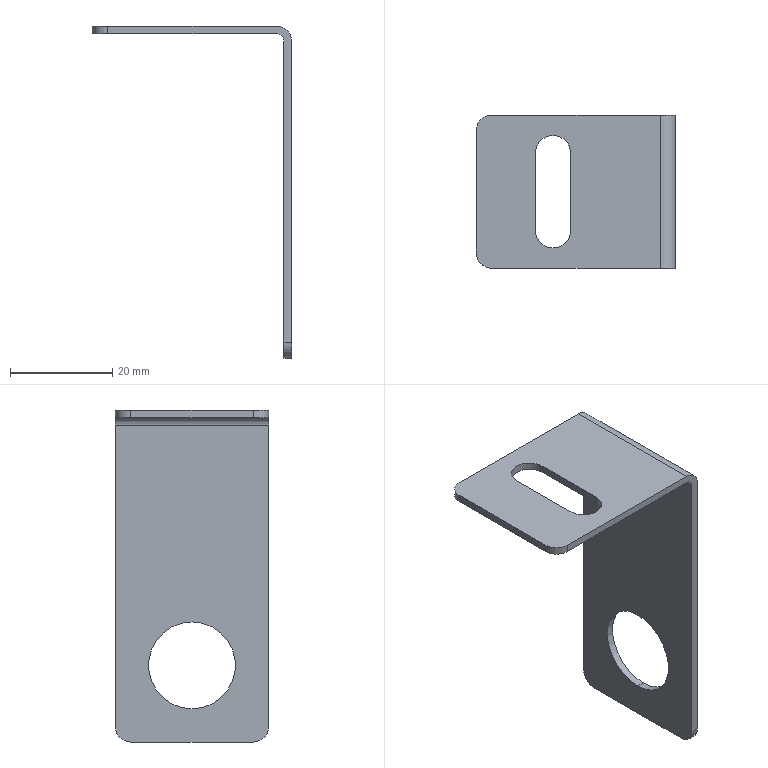Part | SolidWorks | features BaseBody 1 | 1 solid | 20 faces | box 39 x 30 x 65 mm | volume 4002 mm3 | cylinder 10 | plane 10 | commonest cylinder face diameters 6 x5 7 x2 17 x2 3 x1
STEP:
#1=CARTESIAN_POINT('',(18.,0.,-58.5));
#2=VERTEX_POINT('',#1);
#3=CARTESIAN_POINT('',(18.,0.,-41.5));
#4=VERTEX_POINT('',#3);
#5=CARTESIAN_POINT('',(18.,0.,-50.));
#6=DIRECTION('',(-1.,0.,0.));
#7=DIRECTION('',(0.,0.,-1.));
#8=AXIS2_PLACEMENT_3D('',#5,#6,#7);
#9=CIRCLE('',#8,8.5);
#10=EDGE_CURVE('',#2,#4,#9,.T.);
#11=ORIENTED_EDGE('',*,*,#10,.T.);
#12=CARTESIAN_POINT('',(19.5,0.,-41.5));
#13=VERTEX_POINT('',#12);
#14=CARTESIAN_POINT('',(9.5,0.,-41.5));
#15=DIRECTION('',(1.,0.,0.));
#16=VECTOR('',#15,1000.);
#17=LINE('',#14,#16);
#18=EDGE_CURVE('',#4,#13,#17,.T.);
#19=ORIENTED_EDGE('',*,*,#18,.T.);
#20=CARTESIAN_POINT('',(19.5,0.,-58.5));
#21=VERTEX_POINT('',#20);
#22=CARTESIAN_POINT('',(19.5,0.,-50.));
#23=DIRECTION('',(-1.,0.,0.));
#24=DIRECTION('',(0.,0.,-1.));
#25=AXIS2_PLACEMENT_3D('',#22,#23,#24);
#26=CIRCLE('',#25,8.5);
#27=EDGE_CURVE('',#21,#13,#26,.T.);
#28=ORIENTED_EDGE('',*,*,#27,.F.);
#29=CARTESIAN_POINT('',(9.5,0.,-58.5));
#30=DIRECTION('',(1.,0.,0.));
#31=VECTOR('',#30,1000.);
#32=LINE('',#29,#31);
#33=EDGE_CURVE('',#2,#21,#32,.T.);
#34=ORIENTED_EDGE('',*,*,#33,.F.);
#35=EDGE_LOOP('',(#11,#19,#28,#34));
#36=FACE_OUTER_BOUND('',#35,.T.);
#37=CARTESIAN_POINT('',(9.5,0.,-50.));
#38=DIRECTION('',(1.,0.,0.));
#39=DIRECTION('',(0.,0.,-1.));
#40=AXIS2_PLACEMENT_3D('',#37,#38,#39);
#41=CYLINDRICAL_SURFACE('',#40,8.5);
#42=ADVANCED_FACE('',(#36),#41,.F.);
#43=CARTESIAN_POINT('',(18.,12.,-65.));
#44=VERTEX_POINT('',#43);
#45=CARTESIAN_POINT('',(18.,15.,-62.));
#46=VERTEX_POINT('',#45);
#47=CARTESIAN_POINT('',(18.,12.,-62.));
#48=DIRECTION('',(1.,0.,0.));
#49=DIRECTION('',(0.,0.,1.));
#50=AXIS2_PLACEMENT_3D('',#47,#48,#49);
#51=CIRCLE('',#50,3.);
#52=EDGE_CURVE('',#44,#46,#51,.T.);
#53=ORIENTED_EDGE('',*,*,#52,.F.);
#54=CARTESIAN_POINT('',(18.,-12.,-65.));
#55=VERTEX_POINT('',#54);
#56=CARTESIAN_POINT('',(18.,0.,-65.));
#57=DIRECTION('',(0.,1.,0.));
#58=VECTOR('',#57,1000.);
#59=LINE('',#56,#58);
#60=EDGE_CURVE('',#55,#44,#59,.T.);
#61=ORIENTED_EDGE('',*,*,#60,.F.);
#62=CARTESIAN_POINT('',(18.,-15.,-62.));
#63=VERTEX_POINT('',#62);
#64=CARTESIAN_POINT('',(18.,-12.,-62.));
#65=DIRECTION('',(1.,0.,0.));
#66=DIRECTION('',(0.,0.,1.));
#67=AXIS2_PLACEMENT_3D('',#64,#65,#66);
#68=CIRCLE('',#67,3.);
#69=EDGE_CURVE('',#63,#55,#68,.T.);
#70=ORIENTED_EDGE('',*,*,#69,.F.);
#71=CARTESIAN_POINT('',(18.,-15.,-3.));
#72=VERTEX_POINT('',#71);
#73=CARTESIAN_POINT('',(18.,-15.,0.));
#74=DIRECTION('',(0.,0.,-1.));
#75=VECTOR('',#74,1000.);
#76=LINE('',#73,#75);
#77=EDGE_CURVE('',#72,#63,#76,.T.);
#78=ORIENTED_EDGE('',*,*,#77,.F.);
#79=CARTESIAN_POINT('',(18.,15.,-3.));
#80=VERTEX_POINT('',#79);
#81=CARTESIAN_POINT('',(18.,0.,-3.));
#82=DIRECTION('',(0.,-1.,0.));
#83=VECTOR('',#82,1000.);
#84=LINE('',#81,#83);
#85=EDGE_CURVE('',#80,#72,#84,.T.);
#86=ORIENTED_EDGE('',*,*,#85,.F.);
#87=CARTESIAN_POINT('',(18.,15.,0.));
#88=DIRECTION('',(0.,0.,1.));
#89=VECTOR('',#88,1000.);
#90=LINE('',#87,#89);
#91=EDGE_CURVE('',#46,#80,#90,.T.);
#92=ORIENTED_EDGE('',*,*,#91,.F.);
#93=EDGE_LOOP('',(#53,#61,#70,#78,#86,#92));
#94=FACE_OUTER_BOUND('',#93,.T.);
#95=ORIENTED_EDGE('',*,*,#10,.F.);
#96=CARTESIAN_POINT('',(18.,0.,-50.));
#97=DIRECTION('',(-1.,0.,0.));
#98=DIRECTION('',(0.,0.,-1.));
#99=AXIS2_PLACEMENT_3D('',#96,#97,#98);
#100=CIRCLE('',#99,8.5);
#101=EDGE_CURVE('',#4,#2,#100,.T.);
#102=ORIENTED_EDGE('',*,*,#101,.F.);
#103=EDGE_LOOP('',(#95,#102));
#104=FACE_BOUND('',#103,.T.);
#105=CARTESIAN_POINT('',(18.,0.,0.));
#106=DIRECTION('',(1.,0.,0.));
#107=DIRECTION('',(0.,0.,-1.));
#108=AXIS2_PLACEMENT_3D('',#105,#106,#107);
#109=PLANE('',#108);
#110=ADVANCED_FACE('',(#94,#104),#109,.F.);
#111=ORIENTED_EDGE('',*,*,#91,.T.);
#112=CARTESIAN_POINT('',(16.5,15.,-1.5));
#113=VERTEX_POINT('',#112);
#114=CARTESIAN_POINT('',(16.5,15.,-3.));
#115=DIRECTION('',(0.,-1.,0.));
#116=DIRECTION('',(0.,0.,-1.));
#117=AXIS2_PLACEMENT_3D('',#114,#115,#116);
#118=CIRCLE('',#117,1.5);
#119=EDGE_CURVE('',#80,#113,#118,.T.);
#120=ORIENTED_EDGE('',*,*,#119,.T.);
#121=CARTESIAN_POINT('',(-16.5,15.,-1.5));
#122=VERTEX_POINT('',#121);
#123=CARTESIAN_POINT('',(0.,15.,-1.5));
#124=DIRECTION('',(1.,0.,0.));
#125=VECTOR('',#124,1000.);
#126=LINE('',#123,#125);
#127=EDGE_CURVE('',#122,#113,#126,.T.);
#128=ORIENTED_EDGE('',*,*,#127,.F.);
#129=CARTESIAN_POINT('',(-16.5,15.,0.));
#130=VERTEX_POINT('',#129);
#131=CARTESIAN_POINT('',(-16.5,15.,-1.5));
#132=DIRECTION('',(0.,0.,1.));
#133=VECTOR('',#132,1000.);
#134=LINE('',#131,#133);
#135=EDGE_CURVE('',#122,#130,#134,.T.);
#136=ORIENTED_EDGE('',*,*,#135,.T.);
#137=CARTESIAN_POINT('',(16.5,15.,0.));
#138=VERTEX_POINT('',#137);
#139=CARTESIAN_POINT('',(-19.5,15.,0.));
#140=DIRECTION('',(1.,0.,0.));
#141=VECTOR('',#140,1000.);
#142=LINE('',#139,#141);
#143=EDGE_CURVE('',#130,#138,#142,.T.);
#144=ORIENTED_EDGE('',*,*,#143,.T.);
#145=CARTESIAN_POINT('',(19.5,15.,-3.));
#146=VERTEX_POINT('',#145);
#147=CARTESIAN_POINT('',(16.5,15.,-3.));
#148=DIRECTION('',(0.,1.,0.));
#149=DIRECTION('',(0.,0.,-1.));
#150=AXIS2_PLACEMENT_3D('',#147,#148,#149);
#151=CIRCLE('',#150,3.);
#152=EDGE_CURVE('',#138,#146,#151,.T.);
#153=ORIENTED_EDGE('',*,*,#152,.T.);
#154=CARTESIAN_POINT('',(19.5,15.,-62.));
#155=VERTEX_POINT('',#154);
#156=CARTESIAN_POINT('',(19.5,15.,-65.));
#157=DIRECTION('',(0.,0.,-1.));
#158=VECTOR('',#157,1000.);
#159=LINE('',#156,#158);
#160=EDGE_CURVE('',#146,#155,#159,.T.);
#161=ORIENTED_EDGE('',*,*,#160,.T.);
#162=CARTESIAN_POINT('',(19.5,15.,-62.));
#163=DIRECTION('',(-1.,0.,0.));
#164=VECTOR('',#163,1000.);
#165=LINE('',#162,#164);
#166=EDGE_CURVE('',#155,#46,#165,.T.);
#167=ORIENTED_EDGE('',*,*,#166,.T.);
#168=EDGE_LOOP('',(#111,#120,#128,#136,#144,#153,#161,#167));
#169=FACE_OUTER_BOUND('',#168,.T.);
#170=CARTESIAN_POINT('',(19.5,15.,-65.));
#171=DIRECTION('',(0.,1.,0.));
#172=DIRECTION('',(0.,0.,1.));
#173=AXIS2_PLACEMENT_3D('',#170,#171,#172);
#174=PLANE('',#173);
#175=ADVANCED_FACE('',(#169),#174,.T.);
#176=ORIENTED_EDGE('',*,*,#52,.T.);
#177=ORIENTED_EDGE('',*,*,#166,.F.);
#178=CARTESIAN_POINT('',(19.5,12.,-65.));
#179=VERTEX_POINT('',#178);
#180=CARTESIAN_POINT('',(19.5,12.,-62.));
#181=DIRECTION('',(-1.,0.,0.));
#182=DIRECTION('',(0.,0.,1.));
#183=AXIS2_PLACEMENT_3D('',#180,#181,#182);
#184=CIRCLE('',#183,3.);
#185=EDGE_CURVE('',#155,#179,#184,.T.);
#186=ORIENTED_EDGE('',*,*,#185,.T.);
#187=CARTESIAN_POINT('',(19.5,12.,-65.));
#188=DIRECTION('',(-1.,0.,0.));
#189=VECTOR('',#188,1000.);
#190=LINE('',#187,#189);
#191=EDGE_CURVE('',#179,#44,#190,.T.);
#192=ORIENTED_EDGE('',*,*,#191,.T.);
#193=EDGE_LOOP('',(#176,#177,#186,#192));
#194=FACE_OUTER_BOUND('',#193,.T.);
#195=CARTESIAN_POINT('',(19.5,12.,-62.));
#196=DIRECTION('',(-1.,0.,0.));
#197=DIRECTION('',(0.,0.,1.));
#198=AXIS2_PLACEMENT_3D('',#195,#196,#197);
#199=CYLINDRICAL_SURFACE('',#198,3.);
#200=ADVANCED_FACE('',(#194),#199,.T.);
#201=CARTESIAN_POINT('',(19.5,-12.,-65.));
#202=VERTEX_POINT('',#201);
#203=CARTESIAN_POINT('',(19.5,-15.,-65.));
#204=DIRECTION('',(0.,-1.,0.));
#205=VECTOR('',#204,1000.);
#206=LINE('',#203,#205);
#207=EDGE_CURVE('',#179,#202,#206,.T.);
#208=ORIENTED_EDGE('',*,*,#207,.T.);
#209=CARTESIAN_POINT('',(19.5,-12.,-65.));
#210=DIRECTION('',(-1.,0.,0.));
#211=VECTOR('',#210,1000.);
#212=LINE('',#209,#211);
#213=EDGE_CURVE('',#202,#55,#212,.T.);
#214=ORIENTED_EDGE('',*,*,#213,.T.);
#215=ORIENTED_EDGE('',*,*,#60,.T.);
#216=ORIENTED_EDGE('',*,*,#191,.F.);
#217=EDGE_LOOP('',(#208,#214,#215,#216));
#218=FACE_OUTER_BOUND('',#217,.T.);
#219=CARTESIAN_POINT('',(19.5,-15.,-65.));
#220=DIRECTION('',(0.,0.,-1.));
#221=DIRECTION('',(-1.,0.,0.));
#222=AXIS2_PLACEMENT_3D('',#219,#220,#221);
#223=PLANE('',#222);
#224=ADVANCED_FACE('',(#218),#223,.T.);
#225=ORIENTED_EDGE('',*,*,#69,.T.);
#226=ORIENTED_EDGE('',*,*,#213,.F.);
#227=CARTESIAN_POINT('',(19.5,-15.,-62.));
#228=VERTEX_POINT('',#227);
#229=CARTESIAN_POINT('',(19.5,-12.,-62.));
#230=DIRECTION('',(-1.,0.,0.));
#231=DIRECTION('',(0.,0.,1.));
#232=AXIS2_PLACEMENT_3D('',#229,#230,#231);
#233=CIRCLE('',#232,3.);
#234=EDGE_CURVE('',#202,#228,#233,.T.);
#235=ORIENTED_EDGE('',*,*,#234,.T.);
#236=CARTESIAN_POINT('',(19.5,-15.,-62.));
#237=DIRECTION('',(-1.,0.,0.));
#238=VECTOR('',#237,1000.);
#239=LINE('',#236,#238);
#240=EDGE_CURVE('',#228,#63,#239,.T.);
#241=ORIENTED_EDGE('',*,*,#240,.T.);
#242=EDGE_LOOP('',(#225,#226,#235,#241));
#243=FACE_OUTER_BOUND('',#242,.T.);
#244=CARTESIAN_POINT('',(19.5,-12.,-62.));
#245=DIRECTION('',(-1.,0.,0.));
#246=DIRECTION('',(0.,0.,1.));
#247=AXIS2_PLACEMENT_3D('',#244,#245,#246);
#248=CYLINDRICAL_SURFACE('',#247,3.);
#249=ADVANCED_FACE('',(#243),#248,.T.);
#250=CARTESIAN_POINT('',(19.5,-15.,-3.));
#251=VERTEX_POINT('',#250);
#252=CARTESIAN_POINT('',(19.5,-15.,-1.5));
#253=DIRECTION('',(0.,0.,1.));
#254=VECTOR('',#253,1000.);
#255=LINE('',#252,#254);
#256=EDGE_CURVE('',#228,#251,#255,.T.);
#257=ORIENTED_EDGE('',*,*,#256,.T.);
#258=CARTESIAN_POINT('',(16.5,-15.,0.));
#259=VERTEX_POINT('',#258);
#260=CARTESIAN_POINT('',(16.5,-15.,-3.));
#261=DIRECTION('',(0.,1.,0.));
#262=DIRECTION('',(0.,0.,-1.));
#263=AXIS2_PLACEMENT_3D('',#260,#261,#262);
#264=CIRCLE('',#263,3.);
#265=EDGE_CURVE('',#259,#251,#264,.T.);
#266=ORIENTED_EDGE('',*,*,#265,.F.);
#267=CARTESIAN_POINT('',(-16.5,-15.,0.));
#268=VERTEX_POINT('',#267);
#269=CARTESIAN_POINT('',(-19.5,-15.,0.));
#270=DIRECTION('',(-1.,0.,0.));
#271=VECTOR('',#270,1000.);
#272=LINE('',#269,#271);
#273=EDGE_CURVE('',#259,#268,#272,.T.);
#274=ORIENTED_EDGE('',*,*,#273,.T.);
#275=CARTESIAN_POINT('',(-16.5,-15.,-1.5));
#276=VERTEX_POINT('',#275);
#277=CARTESIAN_POINT('',(-16.5,-15.,-1.5));
#278=DIRECTION('',(0.,0.,1.));
#279=VECTOR('',#278,1000.);
#280=LINE('',#277,#279);
#281=EDGE_CURVE('',#276,#268,#280,.T.);
#282=ORIENTED_EDGE('',*,*,#281,.F.);
#283=CARTESIAN_POINT('',(16.5,-15.,-1.5));
#284=VERTEX_POINT('',#283);
#285=CARTESIAN_POINT('',(0.,-15.,-1.5));
#286=DIRECTION('',(-1.,0.,0.));
#287=VECTOR('',#286,1000.);
#288=LINE('',#285,#287);
#289=EDGE_CURVE('',#284,#276,#288,.T.);
#290=ORIENTED_EDGE('',*,*,#289,.F.);
#291=CARTESIAN_POINT('',(16.5,-15.,-3.));
#292=DIRECTION('',(0.,1.,0.));
#293=DIRECTION('',(0.,0.,-1.));
#294=AXIS2_PLACEMENT_3D('',#291,#292,#293);
#295=CIRCLE('',#294,1.5);
#296=EDGE_CURVE('',#284,#72,#295,.T.);
#297=ORIENTED_EDGE('',*,*,#296,.T.);
#298=ORIENTED_EDGE('',*,*,#77,.T.);
#299=ORIENTED_EDGE('',*,*,#240,.F.);
#300=EDGE_LOOP('',(#257,#266,#274,#282,#290,#297,#298,#299));
#301=FACE_OUTER_BOUND('',#300,.T.);
#302=CARTESIAN_POINT('',(19.5,-15.,-1.5));
#303=DIRECTION('',(0.,-1.,0.));
#304=DIRECTION('',(0.,0.,-1.));
#305=AXIS2_PLACEMENT_3D('',#302,#303,#304);
#306=PLANE('',#305);
#307=ADVANCED_FACE('',(#301),#306,.T.);
#308=ORIENTED_EDGE('',*,*,#119,.F.);
#309=ORIENTED_EDGE('',*,*,#85,.T.);
#310=ORIENTED_EDGE('',*,*,#296,.F.);
#311=CARTESIAN_POINT('',(16.5,-15.,-1.5));
#312=DIRECTION('',(0.,-1.,0.));
#313=VECTOR('',#312,1000.);
#314=LINE('',#311,#313);
#315=EDGE_CURVE('',#113,#284,#314,.T.);
#316=ORIENTED_EDGE('',*,*,#315,.F.);
#317=EDGE_LOOP('',(#308,#309,#310,#316));
#318=FACE_OUTER_BOUND('',#317,.T.);
#319=CARTESIAN_POINT('',(16.5,-15.,-3.));
#320=DIRECTION('',(0.,-1.,0.));
#321=DIRECTION('',(0.,0.,-1.));
#322=AXIS2_PLACEMENT_3D('',#319,#320,#321);
#323=CYLINDRICAL_SURFACE('',#322,1.5);
#324=ADVANCED_FACE('',(#318),#323,.F.);
#325=ORIENTED_EDGE('',*,*,#18,.F.);
#326=ORIENTED_EDGE('',*,*,#101,.T.);
#327=ORIENTED_EDGE('',*,*,#33,.T.);
#328=CARTESIAN_POINT('',(19.5,0.,-50.));
#329=DIRECTION('',(-1.,0.,0.));
#330=DIRECTION('',(0.,0.,-1.));
#331=AXIS2_PLACEMENT_3D('',#328,#329,#330);
#332=CIRCLE('',#331,8.5);
#333=EDGE_CURVE('',#13,#21,#332,.T.);
#334=ORIENTED_EDGE('',*,*,#333,.F.);
#335=EDGE_LOOP('',(#325,#326,#327,#334));
#336=FACE_OUTER_BOUND('',#335,.T.);
#337=CARTESIAN_POINT('',(9.5,0.,-50.));
#338=DIRECTION('',(1.,0.,0.));
#339=DIRECTION('',(0.,0.,-1.));
#340=AXIS2_PLACEMENT_3D('',#337,#338,#339);
#341=CYLINDRICAL_SURFACE('',#340,8.5);
#342=ADVANCED_FACE('',(#336),#341,.F.);
#343=ORIENTED_EDGE('',*,*,#256,.F.);
#344=ORIENTED_EDGE('',*,*,#234,.F.);
#345=ORIENTED_EDGE('',*,*,#207,.F.);
#346=ORIENTED_EDGE('',*,*,#185,.F.);
#347=ORIENTED_EDGE('',*,*,#160,.F.);
#348=CARTESIAN_POINT('',(19.5,0.,-3.));
#349=DIRECTION('',(0.,-1.,0.));
#350=VECTOR('',#349,1000.);
#351=LINE('',#348,#350);
#352=EDGE_CURVE('',#146,#251,#351,.T.);
#353=ORIENTED_EDGE('',*,*,#352,.T.);
#354=EDGE_LOOP('',(#343,#344,#345,#346,#347,#353));
#355=FACE_OUTER_BOUND('',#354,.T.);
#356=ORIENTED_EDGE('',*,*,#27,.T.);
#357=ORIENTED_EDGE('',*,*,#333,.T.);
#358=EDGE_LOOP('',(#356,#357));
#359=FACE_BOUND('',#358,.T.);
#360=CARTESIAN_POINT('',(19.5,0.,0.));
#361=DIRECTION('',(1.,0.,0.));
#362=DIRECTION('',(0.,0.,-1.));
#363=AXIS2_PLACEMENT_3D('',#360,#361,#362);
#364=PLANE('',#363);
#365=ADVANCED_FACE('',(#355,#359),#364,.T.);
#366=ORIENTED_EDGE('',*,*,#289,.T.);
#367=CARTESIAN_POINT('',(-19.5,-12.,-1.5));
#368=VERTEX_POINT('',#367);
#369=CARTESIAN_POINT('',(-16.5,-12.,-1.5));
#370=DIRECTION('',(0.,0.,-1.));
#371=DIRECTION('',(1.,0.,0.));
#372=AXIS2_PLACEMENT_3D('',#369,#370,#371);
#373=CIRCLE('',#372,3.);
#374=EDGE_CURVE('',#276,#368,#373,.T.);
#375=ORIENTED_EDGE('',*,*,#374,.T.);
#376=CARTESIAN_POINT('',(-19.5,12.,-1.5));
#377=VERTEX_POINT('',#376);
#378=CARTESIAN_POINT('',(-19.5,0.,-1.5));
#379=DIRECTION('',(0.,1.,0.));
#380=VECTOR('',#379,1000.);
#381=LINE('',#378,#380);
#382=EDGE_CURVE('',#368,#377,#381,.T.);
#383=ORIENTED_EDGE('',*,*,#382,.T.);
#384=CARTESIAN_POINT('',(-16.5,12.,-1.5));
#385=DIRECTION('',(0.,0.,-1.));
#386=DIRECTION('',(1.,0.,0.));
#387=AXIS2_PLACEMENT_3D('',#384,#385,#386);
#388=CIRCLE('',#387,3.);
#389=EDGE_CURVE('',#377,#122,#388,.T.);
#390=ORIENTED_EDGE('',*,*,#389,.T.);
#391=ORIENTED_EDGE('',*,*,#127,.T.);
#392=ORIENTED_EDGE('',*,*,#315,.T.);
#393=EDGE_LOOP('',(#366,#375,#383,#390,#391,#392));
#394=FACE_OUTER_BOUND('',#393,.T.);
#395=CARTESIAN_POINT('',(-8.,-7.5,-1.5));
#396=VERTEX_POINT('',#395);
#397=CARTESIAN_POINT('',(-1.,-7.5,-1.5));
#398=VERTEX_POINT('',#397);
#399=CARTESIAN_POINT('',(-4.5,-7.5,-1.5));
#400=DIRECTION('',(0.,0.,1.));
#401=DIRECTION('',(1.,0.,0.));
#402=AXIS2_PLACEMENT_3D('',#399,#400,#401);
#403=CIRCLE('',#402,3.5);
#404=EDGE_CURVE('',#396,#398,#403,.T.);
#405=ORIENTED_EDGE('',*,*,#404,.T.);
#406=CARTESIAN_POINT('',(-1.,7.5,-1.5));
#407=VERTEX_POINT('',#406);
#408=CARTESIAN_POINT('',(-1.,0.,-1.5));
#409=DIRECTION('',(0.,1.,0.));
#410=VECTOR('',#409,1000.);
#411=LINE('',#408,#410);
#412=EDGE_CURVE('',#398,#407,#411,.T.);
#413=ORIENTED_EDGE('',*,*,#412,.T.);
#414=CARTESIAN_POINT('',(-8.,7.5,-1.5));
#415=VERTEX_POINT('',#414);
#416=CARTESIAN_POINT('',(-4.5,7.5,-1.5));
#417=DIRECTION('',(0.,0.,1.));
#418=DIRECTION('',(1.,0.,0.));
#419=AXIS2_PLACEMENT_3D('',#416,#417,#418);
#420=CIRCLE('',#419,3.5);
#421=EDGE_CURVE('',#407,#415,#420,.T.);
#422=ORIENTED_EDGE('',*,*,#421,.T.);
#423=CARTESIAN_POINT('',(-8.,0.,-1.5));
#424=DIRECTION('',(0.,-1.,0.));
#425=VECTOR('',#424,1000.);
#426=LINE('',#423,#425);
#427=EDGE_CURVE('',#415,#396,#426,.T.);
#428=ORIENTED_EDGE('',*,*,#427,.T.);
#429=EDGE_LOOP('',(#405,#413,#422,#428));
#430=FACE_BOUND('',#429,.T.);
#431=CARTESIAN_POINT('',(0.,0.,-1.5));
#432=DIRECTION('',(0.,0.,-1.));
#433=DIRECTION('',(-1.,0.,0.));
#434=AXIS2_PLACEMENT_3D('',#431,#432,#433);
#435=PLANE('',#434);
#436=ADVANCED_FACE('',(#394,#430),#435,.T.);
#437=ORIENTED_EDGE('',*,*,#352,.F.);
#438=ORIENTED_EDGE('',*,*,#152,.F.);
#439=CARTESIAN_POINT('',(16.5,-15.,0.));
#440=DIRECTION('',(0.,-1.,0.));
#441=VECTOR('',#440,1000.);
#442=LINE('',#439,#441);
#443=EDGE_CURVE('',#138,#259,#442,.T.);
#444=ORIENTED_EDGE('',*,*,#443,.T.);
#445=ORIENTED_EDGE('',*,*,#265,.T.);
#446=EDGE_LOOP('',(#437,#438,#444,#445));
#447=FACE_OUTER_BOUND('',#446,.T.);
#448=CARTESIAN_POINT('',(16.5,-15.,-3.));
#449=DIRECTION('',(0.,-1.,0.));
#450=DIRECTION('',(0.,0.,-1.));
#451=AXIS2_PLACEMENT_3D('',#448,#449,#450);
#452=CYLINDRICAL_SURFACE('',#451,3.);
#453=ADVANCED_FACE('',(#447),#452,.T.);
#454=CARTESIAN_POINT('',(-19.5,-12.,0.));
#455=VERTEX_POINT('',#454);
#456=CARTESIAN_POINT('',(-16.5,-12.,0.));
#457=DIRECTION('',(0.,0.,-1.));
#458=DIRECTION('',(1.,0.,0.));
#459=AXIS2_PLACEMENT_3D('',#456,#457,#458);
#460=CIRCLE('',#459,3.);
#461=EDGE_CURVE('',#268,#455,#460,.T.);
#462=ORIENTED_EDGE('',*,*,#461,.T.);
#463=CARTESIAN_POINT('',(-19.5,-12.,-1.5));
#464=DIRECTION('',(0.,0.,-1.));
#465=VECTOR('',#464,1000.);
#466=LINE('',#463,#465);
#467=EDGE_CURVE('',#455,#368,#466,.T.);
#468=ORIENTED_EDGE('',*,*,#467,.T.);
#469=ORIENTED_EDGE('',*,*,#374,.F.);
#470=ORIENTED_EDGE('',*,*,#281,.T.);
#471=EDGE_LOOP('',(#462,#468,#469,#470));
#472=FACE_OUTER_BOUND('',#471,.T.);
#473=CARTESIAN_POINT('',(-16.5,-12.,-1.5));
#474=DIRECTION('',(0.,0.,1.));
#475=DIRECTION('',(1.,0.,0.));
#476=AXIS2_PLACEMENT_3D('',#473,#474,#475);
#477=CYLINDRICAL_SURFACE('',#476,3.);
#478=ADVANCED_FACE('',(#472),#477,.T.);
#479=CARTESIAN_POINT('',(-19.5,12.,0.));
#480=VERTEX_POINT('',#479);
#481=CARTESIAN_POINT('',(-16.5,12.,0.));
#482=DIRECTION('',(0.,0.,-1.));
#483=DIRECTION('',(1.,0.,0.));
#484=AXIS2_PLACEMENT_3D('',#481,#482,#483);
#485=CIRCLE('',#484,3.);
#486=EDGE_CURVE('',#480,#130,#485,.T.);
#487=ORIENTED_EDGE('',*,*,#486,.T.);
#488=ORIENTED_EDGE('',*,*,#135,.F.);
#489=ORIENTED_EDGE('',*,*,#389,.F.);
#490=CARTESIAN_POINT('',(-19.5,12.,-1.5));
#491=DIRECTION('',(0.,0.,1.));
#492=VECTOR('',#491,1000.);
#493=LINE('',#490,#492);
#494=EDGE_CURVE('',#377,#480,#493,.T.);
#495=ORIENTED_EDGE('',*,*,#494,.T.);
#496=EDGE_LOOP('',(#487,#488,#489,#495));
#497=FACE_OUTER_BOUND('',#496,.T.);
#498=CARTESIAN_POINT('',(-16.5,12.,-1.5));
#499=DIRECTION('',(0.,0.,1.));
#500=DIRECTION('',(1.,0.,0.));
#501=AXIS2_PLACEMENT_3D('',#498,#499,#500);
#502=CYLINDRICAL_SURFACE('',#501,3.);
#503=ADVANCED_FACE('',(#497),#502,.T.);
#504=ORIENTED_EDGE('',*,*,#382,.F.);
#505=ORIENTED_EDGE('',*,*,#467,.F.);
#506=CARTESIAN_POINT('',(-19.5,-15.,0.));
#507=DIRECTION('',(0.,1.,0.));
#508=VECTOR('',#507,1000.);
#509=LINE('',#506,#508);
#510=EDGE_CURVE('',#455,#480,#509,.T.);
#511=ORIENTED_EDGE('',*,*,#510,.T.);
#512=ORIENTED_EDGE('',*,*,#494,.F.);
#513=EDGE_LOOP('',(#504,#505,#511,#512));
#514=FACE_OUTER_BOUND('',#513,.T.);
#515=CARTESIAN_POINT('',(-19.5,-15.,-1.5));
#516=DIRECTION('',(-1.,0.,0.));
#517=DIRECTION('',(0.,0.,1.));
#518=AXIS2_PLACEMENT_3D('',#515,#516,#517);
#519=PLANE('',#518);
#520=ADVANCED_FACE('',(#514),#519,.T.);
#521=CARTESIAN_POINT('',(-1.,-7.5,0.));
#522=VERTEX_POINT('',#521);
#523=CARTESIAN_POINT('',(-1.,-7.5,-10.));
#524=DIRECTION('',(0.,0.,-1.));
#525=VECTOR('',#524,1000.);
#526=LINE('',#523,#525);
#527=EDGE_CURVE('',#522,#398,#526,.T.);
#528=ORIENTED_EDGE('',*,*,#527,.F.);
#529=CARTESIAN_POINT('',(-1.,7.5,0.));
#530=VERTEX_POINT('',#529);
#531=CARTESIAN_POINT('',(-1.,7.5,0.));
#532=DIRECTION('',(0.,-1.,0.));
#533=VECTOR('',#532,1000.);
#534=LINE('',#531,#533);
#535=EDGE_CURVE('',#530,#522,#534,.T.);
#536=ORIENTED_EDGE('',*,*,#535,.F.);
#537=CARTESIAN_POINT('',(-1.,7.5,-10.));
#538=DIRECTION('',(0.,0.,1.));
#539=VECTOR('',#538,1000.);
#540=LINE('',#537,#539);
#541=EDGE_CURVE('',#407,#530,#540,.T.);
#542=ORIENTED_EDGE('',*,*,#541,.F.);
#543=ORIENTED_EDGE('',*,*,#412,.F.);
#544=EDGE_LOOP('',(#528,#536,#542,#543));
#545=FACE_OUTER_BOUND('',#544,.T.);
#546=CARTESIAN_POINT('',(-1.,7.5,-10.));
#547=DIRECTION('',(1.,0.,0.));
#548=DIRECTION('',(0.,1.,0.));
#549=AXIS2_PLACEMENT_3D('',#546,#547,#548);
#550=PLANE('',#549);
#551=ADVANCED_FACE('',(#545),#550,.F.);
#552=CARTESIAN_POINT('',(-8.,-7.5,0.));
#553=VERTEX_POINT('',#552);
#554=CARTESIAN_POINT('',(-8.,-7.5,-10.));
#555=DIRECTION('',(0.,0.,-1.));
#556=VECTOR('',#555,1000.);
#557=LINE('',#554,#556);
#558=EDGE_CURVE('',#553,#396,#557,.T.);
#559=ORIENTED_EDGE('',*,*,#558,.F.);
#560=CARTESIAN_POINT('',(-4.5,-7.5,0.));
#561=DIRECTION('',(0.,0.,-1.));
#562=DIRECTION('',(1.,0.,0.));
#563=AXIS2_PLACEMENT_3D('',#560,#561,#562);
#564=CIRCLE('',#563,3.5);
#565=EDGE_CURVE('',#522,#553,#564,.T.);
#566=ORIENTED_EDGE('',*,*,#565,.F.);
#567=ORIENTED_EDGE('',*,*,#527,.T.);
#568=ORIENTED_EDGE('',*,*,#404,.F.);
#569=EDGE_LOOP('',(#559,#566,#567,#568));
#570=FACE_OUTER_BOUND('',#569,.T.);
#571=CARTESIAN_POINT('',(-4.5,-7.5,-10.));
#572=DIRECTION('',(0.,0.,1.));
#573=DIRECTION('',(1.,0.,0.));
#574=AXIS2_PLACEMENT_3D('',#571,#572,#573);
#575=CYLINDRICAL_SURFACE('',#574,3.5);
#576=ADVANCED_FACE('',(#570),#575,.F.);
#577=CARTESIAN_POINT('',(-8.,7.5,0.));
#578=VERTEX_POINT('',#577);
#579=CARTESIAN_POINT('',(-8.,7.5,-10.));
#580=DIRECTION('',(0.,0.,-1.));
#581=VECTOR('',#580,1000.);
#582=LINE('',#579,#581);
#583=EDGE_CURVE('',#578,#415,#582,.T.);
#584=ORIENTED_EDGE('',*,*,#583,.F.);
#585=CARTESIAN_POINT('',(-8.,7.5,0.));
#586=DIRECTION('',(0.,1.,0.));
#587=VECTOR('',#586,1000.);
#588=LINE('',#585,#587);
#589=EDGE_CURVE('',#553,#578,#588,.T.);
#590=ORIENTED_EDGE('',*,*,#589,.F.);
#591=ORIENTED_EDGE('',*,*,#558,.T.);
#592=ORIENTED_EDGE('',*,*,#427,.F.);
#593=EDGE_LOOP('',(#584,#590,#591,#592));
#594=FACE_OUTER_BOUND('',#593,.T.);
#595=CARTESIAN_POINT('',(-8.,7.5,-10.));
#596=DIRECTION('',(-1.,0.,0.));
#597=DIRECTION('',(0.,-1.,0.));
#598=AXIS2_PLACEMENT_3D('',#595,#596,#597);
#599=PLANE('',#598);
#600=ADVANCED_FACE('',(#594),#599,.F.);
#601=ORIENTED_EDGE('',*,*,#541,.T.);
#602=CARTESIAN_POINT('',(-4.5,7.5,0.));
#603=DIRECTION('',(0.,0.,-1.));
#604=DIRECTION('',(1.,0.,0.));
#605=AXIS2_PLACEMENT_3D('',#602,#603,#604);
#606=CIRCLE('',#605,3.5);
#607=EDGE_CURVE('',#578,#530,#606,.T.);
#608=ORIENTED_EDGE('',*,*,#607,.F.);
#609=ORIENTED_EDGE('',*,*,#583,.T.);
#610=ORIENTED_EDGE('',*,*,#421,.F.);
#611=EDGE_LOOP('',(#601,#608,#609,#610));
#612=FACE_OUTER_BOUND('',#611,.T.);
#613=CARTESIAN_POINT('',(-4.5,7.5,-10.));
#614=DIRECTION('',(0.,0.,1.));
#615=DIRECTION('',(1.,0.,0.));
#616=AXIS2_PLACEMENT_3D('',#613,#614,#615);
#617=CYLINDRICAL_SURFACE('',#616,3.5);
#618=ADVANCED_FACE('',(#612),#617,.F.);
#619=ORIENTED_EDGE('',*,*,#486,.F.);
#620=ORIENTED_EDGE('',*,*,#510,.F.);
#621=ORIENTED_EDGE('',*,*,#461,.F.);
#622=ORIENTED_EDGE('',*,*,#273,.F.);
#623=ORIENTED_EDGE('',*,*,#443,.F.);
#624=ORIENTED_EDGE('',*,*,#143,.F.);
#625=EDGE_LOOP('',(#619,#620,#621,#622,#623,#624));
#626=FACE_OUTER_BOUND('',#625,.T.);
#627=ORIENTED_EDGE('',*,*,#607,.T.);
#628=ORIENTED_EDGE('',*,*,#535,.T.);
#629=ORIENTED_EDGE('',*,*,#565,.T.);
#630=ORIENTED_EDGE('',*,*,#589,.T.);
#631=EDGE_LOOP('',(#627,#628,#629,#630));
#632=FACE_BOUND('',#631,.T.);
#633=CARTESIAN_POINT('',(0.,0.,0.));
#634=DIRECTION('',(0.,0.,-1.));
#635=DIRECTION('',(-1.,0.,0.));
#636=AXIS2_PLACEMENT_3D('',#633,#634,#635);
#637=PLANE('',#636);
#638=ADVANCED_FACE('',(#626,#632),#637,.F.);
#639=CLOSED_SHELL('',(#42,#110,#175,#200,#224,#249,#307,#324,#342,#365,#436,#453,#478,#503,#520,#551,#576,#600,#618,#638));
#640=MANIFOLD_SOLID_BREP('',#639);
#641=CARTESIAN_POINT('',(0.,0.,0.));
#642=DIRECTION('',(0.,0.,1.));
#643=DIRECTION('',(1.,0.,0.));
#644=AXIS2_PLACEMENT_3D('',#641,#642,#643);
#645=(LENGTH_UNIT()NAMED_UNIT(*)SI_UNIT(.MILLI.,.METRE.));
#646=UNCERTAINTY_MEASURE_WITH_UNIT(LENGTH_MEASURE(0.00001),#645,'','');
#647=(NAMED_UNIT(*)PLANE_ANGLE_UNIT()SI_UNIT($,.RADIAN.));
#648=(NAMED_UNIT(*)SI_UNIT($,.STERADIAN.)SOLID_ANGLE_UNIT());
#649=(GEOMETRIC_REPRESENTATION_CONTEXT(3)GLOBAL_UNCERTAINTY_ASSIGNED_CONTEXT((#646))GLOBAL_UNIT_ASSIGNED_CONTEXT((#645,#647,#648))REPRESENTATION_CONTEXT('',''));
#650=ADVANCED_BREP_SHAPE_REPRESENTATION('',(#640,#644),#649);